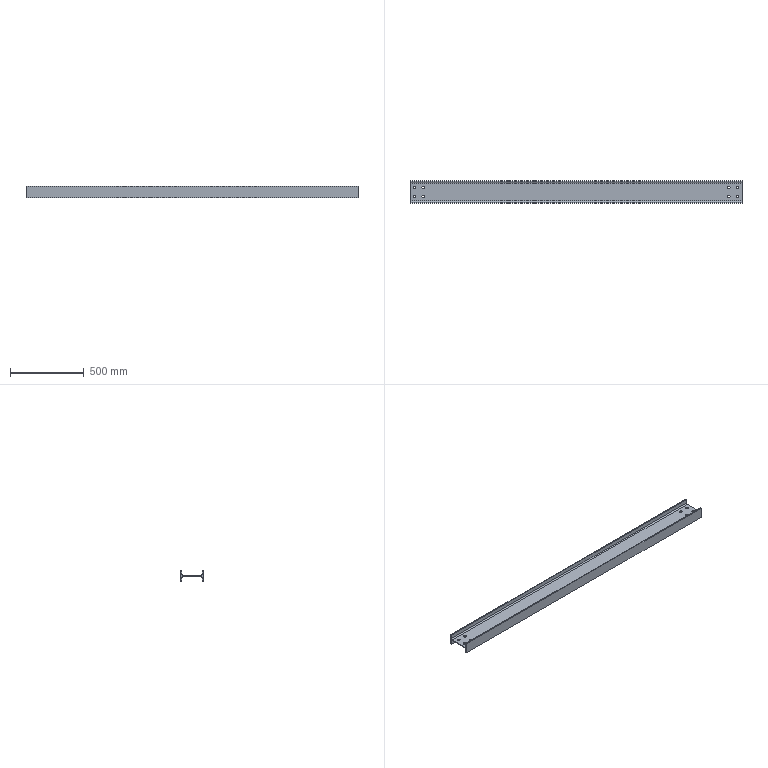Part | STEP file | 粉仓辅梁10主体_Default<As Machined> | 1 solid | 34 faces | box 2255 x 150 x 75 mm | volume 4013694 mm3 | cylinder 20 | plane 14 | commonest cylinder face diameters 19 x16 16 x4